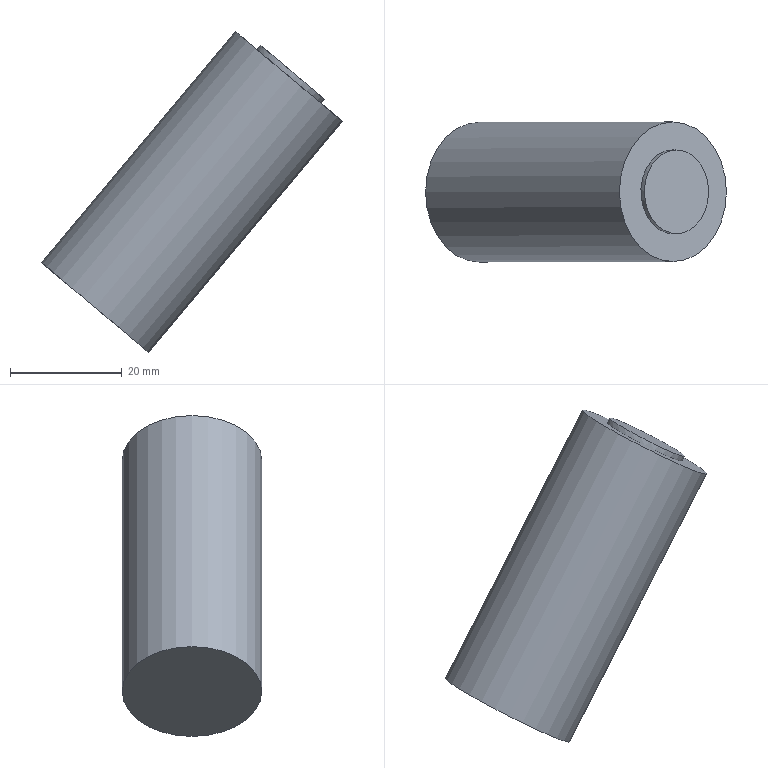Part | NX | features solid 2 | 1 solid | 5 faces | box 53.862 x 25 x 57.436 mm | volume 26684 mm3 | plane 3 | cylinder 2 | commonest cylinder face diameters 15 x1 25 x1
STEP:
#1=CARTESIAN_POINT('',(883.393,-487.5,-114.006));
#2=VERTEX_POINT('',#1);
#3=CARTESIAN_POINT('',(883.393,-500.,-114.006));
#4=DIRECTION('',(0.6428,0.,0.766));
#5=DIRECTION('',(0.,1.,0.));
#6=AXIS2_PLACEMENT_3D('',#3,#4,#5);
#7=CIRCLE('',#6,12.5);
#8=EDGE_CURVE('',#2,#2,#7,.T.);
#9=ORIENTED_EDGE('',*,*,#8,.T.);
#10=EDGE_LOOP('',(#9));
#11=FACE_BOUND('',#10,.T.);
#12=CARTESIAN_POINT('',(883.393,-492.5,-114.006));
#13=VERTEX_POINT('',#12);
#14=CARTESIAN_POINT('',(883.393,-500.,-114.006));
#15=DIRECTION('',(0.6428,0.,0.766));
#16=DIRECTION('',(0.,1.,0.));
#17=AXIS2_PLACEMENT_3D('',#14,#15,#16);
#18=CIRCLE('',#17,7.5);
#19=EDGE_CURVE('',#13,#13,#18,.T.);
#20=ORIENTED_EDGE('',*,*,#19,.F.);
#21=EDGE_LOOP('',(#20));
#22=FACE_BOUND('',#21,.T.);
#23=CARTESIAN_POINT('',(883.393,-500.,-114.006));
#24=DIRECTION('',(0.6428,0.,0.766));
#25=DIRECTION('',(0.,1.,0.));
#26=AXIS2_PLACEMENT_3D('',#23,#24,#25);
#27=PLANE('',#26);
#28=ADVANCED_FACE('',(#11,#22),#27,.T.);
#29=ORIENTED_EDGE('',*,*,#8,.F.);
#30=EDGE_LOOP('',(#29));
#31=FACE_BOUND('',#30,.T.);
#32=CARTESIAN_POINT('',(858.258,-500.,-163.408));
#33=VERTEX_POINT('',#32);
#34=CARTESIAN_POINT('',(848.682,-500.,-155.373));
#35=DIRECTION('',(0.6428,0.,0.766));
#36=DIRECTION('',(0.766,0.,-0.6428));
#37=AXIS2_PLACEMENT_3D('',#34,#35,#36);
#38=CIRCLE('',#37,12.5);
#39=EDGE_CURVE('',#33,#33,#38,.T.);
#40=ORIENTED_EDGE('',*,*,#39,.T.);
#41=EDGE_LOOP('',(#40));
#42=FACE_BOUND('',#41,.T.);
#43=CARTESIAN_POINT('',(884.036,-500.,-113.24));
#44=DIRECTION('',(-0.6428,0.,-0.766));
#45=DIRECTION('',(0.,-1.,0.));
#46=AXIS2_PLACEMENT_3D('',#43,#44,#45);
#47=CYLINDRICAL_SURFACE('',#46,12.5);
#48=ADVANCED_FACE('',(#31,#42),#47,.T.);
#49=ORIENTED_EDGE('',*,*,#39,.F.);
#50=EDGE_LOOP('',(#49));
#51=FACE_BOUND('',#50,.T.);
#52=CARTESIAN_POINT('',(848.682,-500.,-155.373));
#53=DIRECTION('',(0.6428,0.,0.766));
#54=DIRECTION('',(0.,1.,0.));
#55=AXIS2_PLACEMENT_3D('',#52,#53,#54);
#56=PLANE('',#55);
#57=ADVANCED_FACE('',(#51),#56,.F.);
#58=CARTESIAN_POINT('',(889.781,-500.,-118.061));
#59=VERTEX_POINT('',#58);
#60=CARTESIAN_POINT('',(884.036,-500.,-113.24));
#61=DIRECTION('',(0.6428,0.,0.766));
#62=DIRECTION('',(0.766,0.,-0.6428));
#63=AXIS2_PLACEMENT_3D('',#60,#61,#62);
#64=CIRCLE('',#63,7.5);
#65=EDGE_CURVE('',#59,#59,#64,.T.);
#66=ORIENTED_EDGE('',*,*,#65,.F.);
#67=EDGE_LOOP('',(#66));
#68=FACE_BOUND('',#67,.T.);
#69=ORIENTED_EDGE('',*,*,#19,.T.);
#70=EDGE_LOOP('',(#69));
#71=FACE_BOUND('',#70,.T.);
#72=CARTESIAN_POINT('',(889.821,-500.,-106.346));
#73=DIRECTION('',(-0.6428,0.,-0.766));
#74=DIRECTION('',(0.,-1.,0.));
#75=AXIS2_PLACEMENT_3D('',#72,#73,#74);
#76=CYLINDRICAL_SURFACE('',#75,7.5);
#77=ADVANCED_FACE('',(#68,#71),#76,.T.);
#78=ORIENTED_EDGE('',*,*,#65,.T.);
#79=EDGE_LOOP('',(#78));
#80=FACE_BOUND('',#79,.T.);
#81=CARTESIAN_POINT('',(884.036,-500.,-113.24));
#82=DIRECTION('',(0.6428,0.,0.766));
#83=DIRECTION('',(0.,1.,0.));
#84=AXIS2_PLACEMENT_3D('',#81,#82,#83);
#85=PLANE('',#84);
#86=ADVANCED_FACE('',(#80),#85,.T.);
#87=CLOSED_SHELL('',(#28,#48,#57,#77,#86));
#88=MANIFOLD_SOLID_BREP('',#87);
#89=(LENGTH_UNIT()NAMED_UNIT(*)SI_UNIT(.MILLI.,.METRE.));
#90=UNCERTAINTY_MEASURE_WITH_UNIT(LENGTH_MEASURE(0.00001),#89,'','');
#91=(NAMED_UNIT(*)PLANE_ANGLE_UNIT()SI_UNIT($,.RADIAN.));
#92=(NAMED_UNIT(*)SI_UNIT($,.STERADIAN.)SOLID_ANGLE_UNIT());
#93=(GEOMETRIC_REPRESENTATION_CONTEXT(3)GLOBAL_UNCERTAINTY_ASSIGNED_CONTEXT((#90))GLOBAL_UNIT_ASSIGNED_CONTEXT((#89,#91,#92))REPRESENTATION_CONTEXT('',''));
#94=ADVANCED_BREP_SHAPE_REPRESENTATION('',(#88),#93);